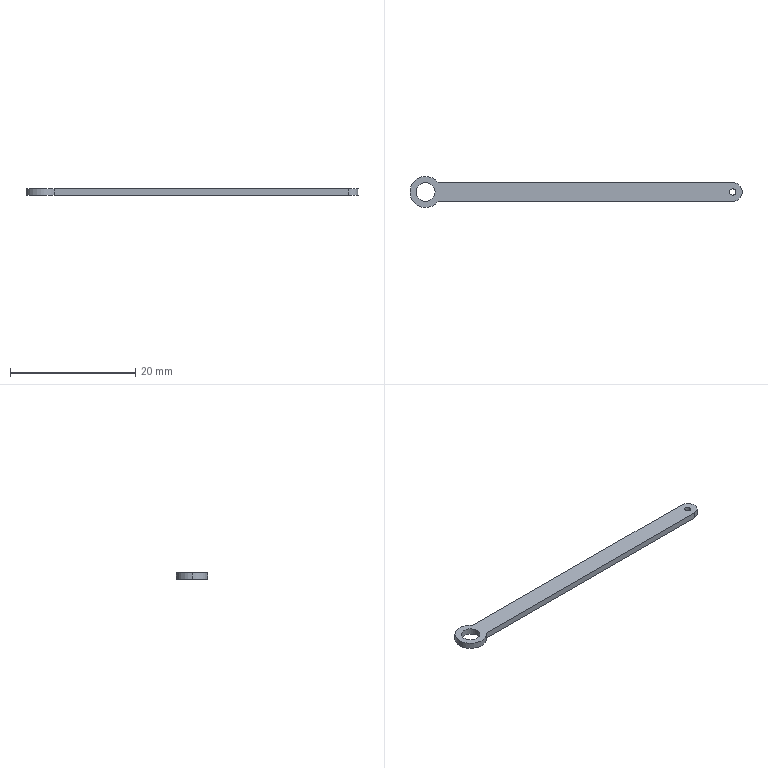Part | SolidWorks | features Extrusion 1 | 1 solid | 11 faces | box 53.128 x 5 x 1 mm | volume 155.677 mm3 | cylinder 7 | plane 4 | commonest cylinder face diameters 3 x3 1 x2 5 x2
STEP:
#1=CARTESIAN_POINT('',(48.628,0.,1.));
#2=VERTEX_POINT('',#1);
#3=CARTESIAN_POINT('',(49.628,0.,1.));
#4=VERTEX_POINT('',#3);
#5=CARTESIAN_POINT('',(49.128,0.,1.));
#6=DIRECTION('',(0.,0.,1.));
#7=DIRECTION('',(1.,0.,0.));
#8=AXIS2_PLACEMENT_3D('',#5,#6,#7);
#9=CIRCLE('',#8,0.5);
#10=EDGE_CURVE('',#2,#4,#9,.T.);
#11=ORIENTED_EDGE('',*,*,#10,.T.);
#12=CARTESIAN_POINT('',(49.628,0.,0.));
#13=VERTEX_POINT('',#12);
#14=CARTESIAN_POINT('',(49.628,0.,1.));
#15=DIRECTION('',(0.,0.,-1.));
#16=VECTOR('',#15,1000.);
#17=LINE('',#14,#16);
#18=EDGE_CURVE('',#4,#13,#17,.T.);
#19=ORIENTED_EDGE('',*,*,#18,.T.);
#20=CARTESIAN_POINT('',(48.628,0.,0.));
#21=VERTEX_POINT('',#20);
#22=CARTESIAN_POINT('',(49.128,0.,0.));
#23=DIRECTION('',(0.,0.,1.));
#24=DIRECTION('',(1.,0.,0.));
#25=AXIS2_PLACEMENT_3D('',#22,#23,#24);
#26=CIRCLE('',#25,0.5);
#27=EDGE_CURVE('',#21,#13,#26,.T.);
#28=ORIENTED_EDGE('',*,*,#27,.F.);
#29=CARTESIAN_POINT('',(48.628,0.,1.));
#30=DIRECTION('',(0.,0.,-1.));
#31=VECTOR('',#30,1000.);
#32=LINE('',#29,#31);
#33=EDGE_CURVE('',#2,#21,#32,.T.);
#34=ORIENTED_EDGE('',*,*,#33,.F.);
#35=EDGE_LOOP('',(#11,#19,#28,#34));
#36=FACE_OUTER_BOUND('',#35,.T.);
#37=CARTESIAN_POINT('',(49.128,0.,1.));
#38=DIRECTION('',(0.,0.,-1.));
#39=DIRECTION('',(-1.,0.,0.));
#40=AXIS2_PLACEMENT_3D('',#37,#38,#39);
#41=CYLINDRICAL_SURFACE('',#40,0.5);
#42=ADVANCED_FACE('',(#36),#41,.F.);
#43=CARTESIAN_POINT('',(-1.5,0.,1.));
#44=VERTEX_POINT('',#43);
#45=CARTESIAN_POINT('',(1.5,0.,1.));
#46=VERTEX_POINT('',#45);
#47=CARTESIAN_POINT('',(0.,0.,1.));
#48=DIRECTION('',(0.,0.,1.));
#49=DIRECTION('',(1.,0.,0.));
#50=AXIS2_PLACEMENT_3D('',#47,#48,#49);
#51=CIRCLE('',#50,1.5);
#52=EDGE_CURVE('',#44,#46,#51,.T.);
#53=ORIENTED_EDGE('',*,*,#52,.T.);
#54=CARTESIAN_POINT('',(1.5,0.,0.));
#55=VERTEX_POINT('',#54);
#56=CARTESIAN_POINT('',(1.5,0.,1.));
#57=DIRECTION('',(0.,0.,-1.));
#58=VECTOR('',#57,1000.);
#59=LINE('',#56,#58);
#60=EDGE_CURVE('',#46,#55,#59,.T.);
#61=ORIENTED_EDGE('',*,*,#60,.T.);
#62=CARTESIAN_POINT('',(-1.5,0.,0.));
#63=VERTEX_POINT('',#62);
#64=CARTESIAN_POINT('',(0.,0.,0.));
#65=DIRECTION('',(0.,0.,1.));
#66=DIRECTION('',(1.,0.,0.));
#67=AXIS2_PLACEMENT_3D('',#64,#65,#66);
#68=CIRCLE('',#67,1.5);
#69=EDGE_CURVE('',#63,#55,#68,.T.);
#70=ORIENTED_EDGE('',*,*,#69,.F.);
#71=CARTESIAN_POINT('',(-1.5,0.,1.));
#72=DIRECTION('',(0.,0.,-1.));
#73=VECTOR('',#72,1000.);
#74=LINE('',#71,#73);
#75=EDGE_CURVE('',#44,#63,#74,.T.);
#76=ORIENTED_EDGE('',*,*,#75,.F.);
#77=EDGE_LOOP('',(#53,#61,#70,#76));
#78=FACE_OUTER_BOUND('',#77,.T.);
#79=CARTESIAN_POINT('',(0.,0.,1.));
#80=DIRECTION('',(0.,0.,-1.));
#81=DIRECTION('',(-1.,0.,0.));
#82=AXIS2_PLACEMENT_3D('',#79,#80,#81);
#83=CYLINDRICAL_SURFACE('',#82,1.5);
#84=ADVANCED_FACE('',(#78),#83,.F.);
#85=CARTESIAN_POINT('',(-2.5,0.,1.));
#86=VERTEX_POINT('',#85);
#87=CARTESIAN_POINT('',(2.,-1.5,1.));
#88=VERTEX_POINT('',#87);
#89=CARTESIAN_POINT('',(0.,0.,1.));
#90=DIRECTION('',(0.,0.,1.));
#91=DIRECTION('',(1.,0.,0.));
#92=AXIS2_PLACEMENT_3D('',#89,#90,#91);
#93=CIRCLE('',#92,2.5);
#94=EDGE_CURVE('',#86,#88,#93,.T.);
#95=ORIENTED_EDGE('',*,*,#94,.F.);
#96=CARTESIAN_POINT('',(-2.5,0.,0.));
#97=VERTEX_POINT('',#96);
#98=CARTESIAN_POINT('',(-2.5,0.,1.));
#99=DIRECTION('',(0.,0.,-1.));
#100=VECTOR('',#99,1000.);
#101=LINE('',#98,#100);
#102=EDGE_CURVE('',#86,#97,#101,.T.);
#103=ORIENTED_EDGE('',*,*,#102,.T.);
#104=CARTESIAN_POINT('',(2.,-1.5,0.));
#105=VERTEX_POINT('',#104);
#106=CARTESIAN_POINT('',(0.,0.,0.));
#107=DIRECTION('',(0.,0.,1.));
#108=DIRECTION('',(1.,0.,0.));
#109=AXIS2_PLACEMENT_3D('',#106,#107,#108);
#110=CIRCLE('',#109,2.5);
#111=EDGE_CURVE('',#97,#105,#110,.T.);
#112=ORIENTED_EDGE('',*,*,#111,.T.);
#113=CARTESIAN_POINT('',(2.,-1.5,1.));
#114=DIRECTION('',(0.,0.,-1.));
#115=VECTOR('',#114,1000.);
#116=LINE('',#113,#115);
#117=EDGE_CURVE('',#88,#105,#116,.T.);
#118=ORIENTED_EDGE('',*,*,#117,.F.);
#119=EDGE_LOOP('',(#95,#103,#112,#118));
#120=FACE_OUTER_BOUND('',#119,.T.);
#121=CARTESIAN_POINT('',(0.,0.,1.));
#122=DIRECTION('',(0.,0.,-1.));
#123=DIRECTION('',(-1.,0.,0.));
#124=AXIS2_PLACEMENT_3D('',#121,#122,#123);
#125=CYLINDRICAL_SURFACE('',#124,2.5);
#126=ADVANCED_FACE('',(#120),#125,.T.);
#127=ORIENTED_EDGE('',*,*,#52,.F.);
#128=CARTESIAN_POINT('',(0.,0.,1.));
#129=DIRECTION('',(0.,0.,1.));
#130=DIRECTION('',(1.,0.,0.));
#131=AXIS2_PLACEMENT_3D('',#128,#129,#130);
#132=CIRCLE('',#131,1.5);
#133=EDGE_CURVE('',#46,#44,#132,.T.);
#134=ORIENTED_EDGE('',*,*,#133,.F.);
#135=EDGE_LOOP('',(#127,#134));
#136=FACE_BOUND('',#135,.T.);
#137=CARTESIAN_POINT('',(49.128,-1.5,1.));
#138=VERTEX_POINT('',#137);
#139=CARTESIAN_POINT('',(49.128,1.5,1.));
#140=VERTEX_POINT('',#139);
#141=CARTESIAN_POINT('',(49.128,0.,1.));
#142=DIRECTION('',(0.,0.,1.));
#143=DIRECTION('',(1.,0.,0.));
#144=AXIS2_PLACEMENT_3D('',#141,#142,#143);
#145=CIRCLE('',#144,1.5);
#146=EDGE_CURVE('',#138,#140,#145,.T.);
#147=ORIENTED_EDGE('',*,*,#146,.T.);
#148=CARTESIAN_POINT('',(2.,1.5,1.));
#149=VERTEX_POINT('',#148);
#150=CARTESIAN_POINT('',(49.128,1.5,1.));
#151=DIRECTION('',(-1.,0.,0.));
#152=VECTOR('',#151,1000.);
#153=LINE('',#150,#152);
#154=EDGE_CURVE('',#140,#149,#153,.T.);
#155=ORIENTED_EDGE('',*,*,#154,.T.);
#156=CARTESIAN_POINT('',(0.,0.,1.));
#157=DIRECTION('',(0.,0.,1.));
#158=DIRECTION('',(1.,0.,0.));
#159=AXIS2_PLACEMENT_3D('',#156,#157,#158);
#160=CIRCLE('',#159,2.5);
#161=EDGE_CURVE('',#149,#86,#160,.T.);
#162=ORIENTED_EDGE('',*,*,#161,.T.);
#163=ORIENTED_EDGE('',*,*,#94,.T.);
#164=CARTESIAN_POINT('',(2.,-1.5,1.));
#165=DIRECTION('',(1.,0.,0.));
#166=VECTOR('',#165,1000.);
#167=LINE('',#164,#166);
#168=EDGE_CURVE('',#88,#138,#167,.T.);
#169=ORIENTED_EDGE('',*,*,#168,.T.);
#170=EDGE_LOOP('',(#147,#155,#162,#163,#169));
#171=FACE_OUTER_BOUND('',#170,.T.);
#172=ORIENTED_EDGE('',*,*,#10,.F.);
#173=CARTESIAN_POINT('',(49.128,0.,1.));
#174=DIRECTION('',(0.,0.,1.));
#175=DIRECTION('',(1.,0.,0.));
#176=AXIS2_PLACEMENT_3D('',#173,#174,#175);
#177=CIRCLE('',#176,0.5);
#178=EDGE_CURVE('',#4,#2,#177,.T.);
#179=ORIENTED_EDGE('',*,*,#178,.F.);
#180=EDGE_LOOP('',(#172,#179));
#181=FACE_BOUND('',#180,.T.);
#182=CARTESIAN_POINT('',(49.128,0.,1.));
#183=DIRECTION('',(0.,0.,1.));
#184=DIRECTION('',(1.,0.,0.));
#185=AXIS2_PLACEMENT_3D('',#182,#183,#184);
#186=PLANE('',#185);
#187=ADVANCED_FACE('',(#136,#171,#181),#186,.T.);
#188=CARTESIAN_POINT('',(49.128,-1.5,0.));
#189=VERTEX_POINT('',#188);
#190=CARTESIAN_POINT('',(49.128,1.5,0.));
#191=VERTEX_POINT('',#190);
#192=CARTESIAN_POINT('',(49.128,0.,0.));
#193=DIRECTION('',(0.,0.,1.));
#194=DIRECTION('',(1.,0.,0.));
#195=AXIS2_PLACEMENT_3D('',#192,#193,#194);
#196=CIRCLE('',#195,1.5);
#197=EDGE_CURVE('',#189,#191,#196,.T.);
#198=ORIENTED_EDGE('',*,*,#197,.F.);
#199=CARTESIAN_POINT('',(2.,-1.5,0.));
#200=DIRECTION('',(1.,0.,0.));
#201=VECTOR('',#200,1000.);
#202=LINE('',#199,#201);
#203=EDGE_CURVE('',#105,#189,#202,.T.);
#204=ORIENTED_EDGE('',*,*,#203,.F.);
#205=ORIENTED_EDGE('',*,*,#111,.F.);
#206=CARTESIAN_POINT('',(2.,1.5,0.));
#207=VERTEX_POINT('',#206);
#208=CARTESIAN_POINT('',(0.,0.,0.));
#209=DIRECTION('',(0.,0.,1.));
#210=DIRECTION('',(1.,0.,0.));
#211=AXIS2_PLACEMENT_3D('',#208,#209,#210);
#212=CIRCLE('',#211,2.5);
#213=EDGE_CURVE('',#207,#97,#212,.T.);
#214=ORIENTED_EDGE('',*,*,#213,.F.);
#215=CARTESIAN_POINT('',(49.128,1.5,0.));
#216=DIRECTION('',(-1.,0.,0.));
#217=VECTOR('',#216,1000.);
#218=LINE('',#215,#217);
#219=EDGE_CURVE('',#191,#207,#218,.T.);
#220=ORIENTED_EDGE('',*,*,#219,.F.);
#221=EDGE_LOOP('',(#198,#204,#205,#214,#220));
#222=FACE_OUTER_BOUND('',#221,.T.);
#223=ORIENTED_EDGE('',*,*,#69,.T.);
#224=CARTESIAN_POINT('',(0.,0.,0.));
#225=DIRECTION('',(0.,0.,1.));
#226=DIRECTION('',(1.,0.,0.));
#227=AXIS2_PLACEMENT_3D('',#224,#225,#226);
#228=CIRCLE('',#227,1.5);
#229=EDGE_CURVE('',#55,#63,#228,.T.);
#230=ORIENTED_EDGE('',*,*,#229,.T.);
#231=EDGE_LOOP('',(#223,#230));
#232=FACE_BOUND('',#231,.T.);
#233=ORIENTED_EDGE('',*,*,#27,.T.);
#234=CARTESIAN_POINT('',(49.128,0.,0.));
#235=DIRECTION('',(0.,0.,1.));
#236=DIRECTION('',(1.,0.,0.));
#237=AXIS2_PLACEMENT_3D('',#234,#235,#236);
#238=CIRCLE('',#237,0.5);
#239=EDGE_CURVE('',#13,#21,#238,.T.);
#240=ORIENTED_EDGE('',*,*,#239,.T.);
#241=EDGE_LOOP('',(#233,#240));
#242=FACE_BOUND('',#241,.T.);
#243=CARTESIAN_POINT('',(49.128,0.,0.));
#244=DIRECTION('',(0.,0.,1.));
#245=DIRECTION('',(1.,0.,0.));
#246=AXIS2_PLACEMENT_3D('',#243,#244,#245);
#247=PLANE('',#246);
#248=ADVANCED_FACE('',(#222,#232,#242),#247,.F.);
#249=ORIENTED_EDGE('',*,*,#197,.T.);
#250=CARTESIAN_POINT('',(49.128,1.5,1.));
#251=DIRECTION('',(0.,0.,-1.));
#252=VECTOR('',#251,1000.);
#253=LINE('',#250,#252);
#254=EDGE_CURVE('',#140,#191,#253,.T.);
#255=ORIENTED_EDGE('',*,*,#254,.F.);
#256=ORIENTED_EDGE('',*,*,#146,.F.);
#257=CARTESIAN_POINT('',(49.128,-1.5,1.));
#258=DIRECTION('',(0.,0.,-1.));
#259=VECTOR('',#258,1000.);
#260=LINE('',#257,#259);
#261=EDGE_CURVE('',#138,#189,#260,.T.);
#262=ORIENTED_EDGE('',*,*,#261,.T.);
#263=EDGE_LOOP('',(#249,#255,#256,#262));
#264=FACE_OUTER_BOUND('',#263,.T.);
#265=CARTESIAN_POINT('',(49.128,0.,1.));
#266=DIRECTION('',(0.,0.,-1.));
#267=DIRECTION('',(-1.,0.,0.));
#268=AXIS2_PLACEMENT_3D('',#265,#266,#267);
#269=CYLINDRICAL_SURFACE('',#268,1.5);
#270=ADVANCED_FACE('',(#264),#269,.T.);
#271=ORIENTED_EDGE('',*,*,#219,.T.);
#272=CARTESIAN_POINT('',(2.,1.5,1.));
#273=DIRECTION('',(0.,0.,-1.));
#274=VECTOR('',#273,1000.);
#275=LINE('',#272,#274);
#276=EDGE_CURVE('',#149,#207,#275,.T.);
#277=ORIENTED_EDGE('',*,*,#276,.F.);
#278=ORIENTED_EDGE('',*,*,#154,.F.);
#279=ORIENTED_EDGE('',*,*,#254,.T.);
#280=EDGE_LOOP('',(#271,#277,#278,#279));
#281=FACE_OUTER_BOUND('',#280,.T.);
#282=CARTESIAN_POINT('',(49.128,1.5,1.));
#283=DIRECTION('',(0.,-1.,0.));
#284=DIRECTION('',(1.,0.,0.));
#285=AXIS2_PLACEMENT_3D('',#282,#283,#284);
#286=PLANE('',#285);
#287=ADVANCED_FACE('',(#281),#286,.F.);
#288=ORIENTED_EDGE('',*,*,#102,.F.);
#289=ORIENTED_EDGE('',*,*,#161,.F.);
#290=ORIENTED_EDGE('',*,*,#276,.T.);
#291=ORIENTED_EDGE('',*,*,#213,.T.);
#292=EDGE_LOOP('',(#288,#289,#290,#291));
#293=FACE_OUTER_BOUND('',#292,.T.);
#294=CARTESIAN_POINT('',(0.,0.,1.));
#295=DIRECTION('',(0.,0.,-1.));
#296=DIRECTION('',(-1.,0.,0.));
#297=AXIS2_PLACEMENT_3D('',#294,#295,#296);
#298=CYLINDRICAL_SURFACE('',#297,2.5);
#299=ADVANCED_FACE('',(#293),#298,.T.);
#300=ORIENTED_EDGE('',*,*,#203,.T.);
#301=ORIENTED_EDGE('',*,*,#261,.F.);
#302=ORIENTED_EDGE('',*,*,#168,.F.);
#303=ORIENTED_EDGE('',*,*,#117,.T.);
#304=EDGE_LOOP('',(#300,#301,#302,#303));
#305=FACE_OUTER_BOUND('',#304,.T.);
#306=CARTESIAN_POINT('',(2.,-1.5,1.));
#307=DIRECTION('',(0.,1.,0.));
#308=DIRECTION('',(-1.,0.,0.));
#309=AXIS2_PLACEMENT_3D('',#306,#307,#308);
#310=PLANE('',#309);
#311=ADVANCED_FACE('',(#305),#310,.F.);
#312=ORIENTED_EDGE('',*,*,#60,.F.);
#313=ORIENTED_EDGE('',*,*,#133,.T.);
#314=ORIENTED_EDGE('',*,*,#75,.T.);
#315=ORIENTED_EDGE('',*,*,#229,.F.);
#316=EDGE_LOOP('',(#312,#313,#314,#315));
#317=FACE_OUTER_BOUND('',#316,.T.);
#318=CARTESIAN_POINT('',(0.,0.,1.));
#319=DIRECTION('',(0.,0.,-1.));
#320=DIRECTION('',(-1.,0.,0.));
#321=AXIS2_PLACEMENT_3D('',#318,#319,#320);
#322=CYLINDRICAL_SURFACE('',#321,1.5);
#323=ADVANCED_FACE('',(#317),#322,.F.);
#324=ORIENTED_EDGE('',*,*,#18,.F.);
#325=ORIENTED_EDGE('',*,*,#178,.T.);
#326=ORIENTED_EDGE('',*,*,#33,.T.);
#327=ORIENTED_EDGE('',*,*,#239,.F.);
#328=EDGE_LOOP('',(#324,#325,#326,#327));
#329=FACE_OUTER_BOUND('',#328,.T.);
#330=CARTESIAN_POINT('',(49.128,0.,1.));
#331=DIRECTION('',(0.,0.,-1.));
#332=DIRECTION('',(-1.,0.,0.));
#333=AXIS2_PLACEMENT_3D('',#330,#331,#332);
#334=CYLINDRICAL_SURFACE('',#333,0.5);
#335=ADVANCED_FACE('',(#329),#334,.F.);
#336=CLOSED_SHELL('',(#42,#84,#126,#187,#248,#270,#287,#299,#311,#323,#335));
#337=MANIFOLD_SOLID_BREP('',#336);
#338=CARTESIAN_POINT('',(0.,0.,0.));
#339=DIRECTION('',(0.,0.,1.));
#340=DIRECTION('',(1.,0.,0.));
#341=AXIS2_PLACEMENT_3D('',#338,#339,#340);
#342=(LENGTH_UNIT()NAMED_UNIT(*)SI_UNIT(.MILLI.,.METRE.));
#343=UNCERTAINTY_MEASURE_WITH_UNIT(LENGTH_MEASURE(0.00001),#342,'','');
#344=(NAMED_UNIT(*)PLANE_ANGLE_UNIT()SI_UNIT($,.RADIAN.));
#345=(NAMED_UNIT(*)SI_UNIT($,.STERADIAN.)SOLID_ANGLE_UNIT());
#346=(GEOMETRIC_REPRESENTATION_CONTEXT(3)GLOBAL_UNCERTAINTY_ASSIGNED_CONTEXT((#343))GLOBAL_UNIT_ASSIGNED_CONTEXT((#342,#344,#345))REPRESENTATION_CONTEXT('',''));
#347=ADVANCED_BREP_SHAPE_REPRESENTATION('',(#337,#341),#346);